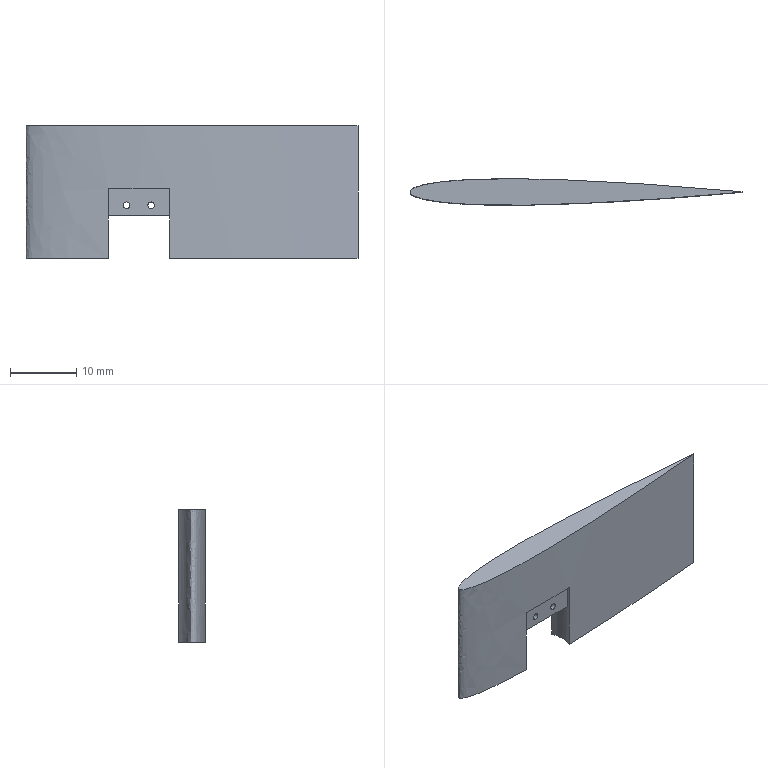Part | SolidWorks | features ICE 3, CurveInFile 1, Extrusion 1 | 1 solid | 17 faces | box 50 x 4.001 x 20 mm | volume 2418 mm3 | plane 9 | cylinder 7 | spline 1 | commonest cylinder face diameters 1 x4 10 x3